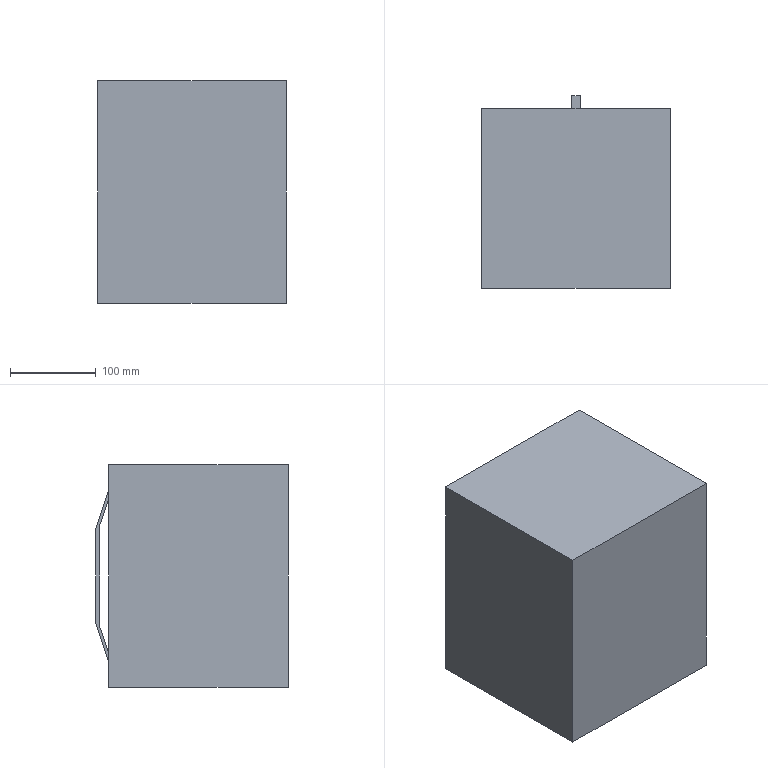Part | SolidWorks | features BaseBody 1 | 1 solid | 14 faces | box 220 x 225 x 260 mm | volume 12020250 mm3 | plane 14
STEP:
#1=CARTESIAN_POINT('',(-5.,120.,55.));
#2=VERTEX_POINT('',#1);
#3=CARTESIAN_POINT('',(5.,120.,55.));
#4=VERTEX_POINT('',#3);
#5=CARTESIAN_POINT('',(5.,120.,55.));
#6=DIRECTION('',(1.,0.,0.));
#7=VECTOR('',#6,1000.);
#8=LINE('',#5,#7);
#9=EDGE_CURVE('',#2,#4,#8,.T.);
#10=ORIENTED_EDGE('',*,*,#9,.T.);
#11=CARTESIAN_POINT('',(5.,120.,-55.));
#12=VERTEX_POINT('',#11);
#13=CARTESIAN_POINT('',(5.,120.,0.));
#14=DIRECTION('',(0.,0.,-1.));
#15=VECTOR('',#14,1000.);
#16=LINE('',#13,#15);
#17=EDGE_CURVE('',#4,#12,#16,.T.);
#18=ORIENTED_EDGE('',*,*,#17,.T.);
#19=CARTESIAN_POINT('',(-5.,120.,-55.));
#20=VERTEX_POINT('',#19);
#21=CARTESIAN_POINT('',(5.,120.,-55.));
#22=DIRECTION('',(-1.,0.,0.));
#23=VECTOR('',#22,1000.);
#24=LINE('',#21,#23);
#25=EDGE_CURVE('',#12,#20,#24,.T.);
#26=ORIENTED_EDGE('',*,*,#25,.T.);
#27=CARTESIAN_POINT('',(-5.,120.,0.));
#28=DIRECTION('',(0.,0.,-1.));
#29=VECTOR('',#28,1000.);
#30=LINE('',#27,#29);
#31=EDGE_CURVE('',#2,#20,#30,.T.);
#32=ORIENTED_EDGE('',*,*,#31,.F.);
#33=EDGE_LOOP('',(#10,#18,#26,#32));
#34=FACE_OUTER_BOUND('',#33,.T.);
#35=CARTESIAN_POINT('',(5.,120.,55.));
#36=DIRECTION('',(0.,-1.,0.));
#37=DIRECTION('',(0.,0.,-1.));
#38=AXIS2_PLACEMENT_3D('',#35,#36,#37);
#39=PLANE('',#38);
#40=ADVANCED_FACE('',(#34),#39,.F.);
#41=CARTESIAN_POINT('',(-5.,115.,-60.));
#42=VERTEX_POINT('',#41);
#43=CARTESIAN_POINT('',(5.,115.,-60.));
#44=VERTEX_POINT('',#43);
#45=CARTESIAN_POINT('',(5.,115.,-60.));
#46=DIRECTION('',(1.,0.,0.));
#47=VECTOR('',#46,1000.);
#48=LINE('',#45,#47);
#49=EDGE_CURVE('',#42,#44,#48,.T.);
#50=ORIENTED_EDGE('',*,*,#49,.T.);
#51=CARTESIAN_POINT('',(5.,115.,60.));
#52=VERTEX_POINT('',#51);
#53=CARTESIAN_POINT('',(5.,115.,0.));
#54=DIRECTION('',(0.,0.,1.));
#55=VECTOR('',#54,1000.);
#56=LINE('',#53,#55);
#57=EDGE_CURVE('',#44,#52,#56,.T.);
#58=ORIENTED_EDGE('',*,*,#57,.T.);
#59=CARTESIAN_POINT('',(-5.,115.,60.));
#60=VERTEX_POINT('',#59);
#61=CARTESIAN_POINT('',(5.,115.,60.));
#62=DIRECTION('',(-1.,0.,0.));
#63=VECTOR('',#62,1000.);
#64=LINE('',#61,#63);
#65=EDGE_CURVE('',#52,#60,#64,.T.);
#66=ORIENTED_EDGE('',*,*,#65,.T.);
#67=CARTESIAN_POINT('',(-5.,115.,0.));
#68=DIRECTION('',(0.,0.,1.));
#69=VECTOR('',#68,1000.);
#70=LINE('',#67,#69);
#71=EDGE_CURVE('',#42,#60,#70,.T.);
#72=ORIENTED_EDGE('',*,*,#71,.F.);
#73=EDGE_LOOP('',(#50,#58,#66,#72));
#74=FACE_OUTER_BOUND('',#73,.T.);
#75=CARTESIAN_POINT('',(5.,115.,-60.));
#76=DIRECTION('',(0.,1.,0.));
#77=DIRECTION('',(0.,0.,-1.));
#78=AXIS2_PLACEMENT_3D('',#75,#76,#77);
#79=PLANE('',#78);
#80=ADVANCED_FACE('',(#74),#79,.F.);
#81=ORIENTED_EDGE('',*,*,#25,.F.);
#82=CARTESIAN_POINT('',(5.,105.,-100.));
#83=VERTEX_POINT('',#82);
#84=CARTESIAN_POINT('',(5.,120.,-55.));
#85=DIRECTION('',(0.,-0.3162,-0.9487));
#86=VECTOR('',#85,1000.);
#87=LINE('',#84,#86);
#88=EDGE_CURVE('',#12,#83,#87,.T.);
#89=ORIENTED_EDGE('',*,*,#88,.T.);
#90=CARTESIAN_POINT('',(-5.,105.,-100.));
#91=VERTEX_POINT('',#90);
#92=CARTESIAN_POINT('',(-110.,105.,-100.));
#93=DIRECTION('',(-1.,0.,0.));
#94=VECTOR('',#93,1000.);
#95=LINE('',#92,#94);
#96=EDGE_CURVE('',#83,#91,#95,.T.);
#97=ORIENTED_EDGE('',*,*,#96,.T.);
#98=CARTESIAN_POINT('',(-5.,120.,-55.));
#99=DIRECTION('',(0.,-0.3162,-0.9487));
#100=VECTOR('',#99,1000.);
#101=LINE('',#98,#100);
#102=EDGE_CURVE('',#20,#91,#101,.T.);
#103=ORIENTED_EDGE('',*,*,#102,.F.);
#104=EDGE_LOOP('',(#81,#89,#97,#103));
#105=FACE_OUTER_BOUND('',#104,.T.);
#106=CARTESIAN_POINT('',(5.,120.,-55.));
#107=DIRECTION('',(0.,-0.9487,0.3162));
#108=DIRECTION('',(-1.,0.,0.));
#109=AXIS2_PLACEMENT_3D('',#106,#107,#108);
#110=PLANE('',#109);
#111=ADVANCED_FACE('',(#105),#110,.F.);
#112=CARTESIAN_POINT('',(-5.,105.,-90.));
#113=VERTEX_POINT('',#112);
#114=CARTESIAN_POINT('',(5.,105.,-90.));
#115=VERTEX_POINT('',#114);
#116=CARTESIAN_POINT('',(-110.,105.,-90.));
#117=DIRECTION('',(1.,0.,0.));
#118=VECTOR('',#117,1000.);
#119=LINE('',#116,#118);
#120=EDGE_CURVE('',#113,#115,#119,.T.);
#121=ORIENTED_EDGE('',*,*,#120,.T.);
#122=CARTESIAN_POINT('',(5.,105.,-90.));
#123=DIRECTION('',(0.,0.3162,0.9487));
#124=VECTOR('',#123,1000.);
#125=LINE('',#122,#124);
#126=EDGE_CURVE('',#115,#44,#125,.T.);
#127=ORIENTED_EDGE('',*,*,#126,.T.);
#128=ORIENTED_EDGE('',*,*,#49,.F.);
#129=CARTESIAN_POINT('',(-5.,105.,-90.));
#130=DIRECTION('',(0.,0.3162,0.9487));
#131=VECTOR('',#130,1000.);
#132=LINE('',#129,#131);
#133=EDGE_CURVE('',#113,#42,#132,.T.);
#134=ORIENTED_EDGE('',*,*,#133,.F.);
#135=EDGE_LOOP('',(#121,#127,#128,#134));
#136=FACE_OUTER_BOUND('',#135,.T.);
#137=CARTESIAN_POINT('',(5.,105.,-90.));
#138=DIRECTION('',(0.,0.9487,-0.3162));
#139=DIRECTION('',(-1.,0.,0.));
#140=AXIS2_PLACEMENT_3D('',#137,#138,#139);
#141=PLANE('',#140);
#142=ADVANCED_FACE('',(#136),#141,.F.);
#143=ORIENTED_EDGE('',*,*,#65,.F.);
#144=CARTESIAN_POINT('',(5.,105.,90.));
#145=VERTEX_POINT('',#144);
#146=CARTESIAN_POINT('',(5.,115.,60.));
#147=DIRECTION('',(0.,-0.3162,0.9487));
#148=VECTOR('',#147,1000.);
#149=LINE('',#146,#148);
#150=EDGE_CURVE('',#52,#145,#149,.T.);
#151=ORIENTED_EDGE('',*,*,#150,.T.);
#152=CARTESIAN_POINT('',(-5.,105.,90.));
#153=VERTEX_POINT('',#152);
#154=CARTESIAN_POINT('',(-110.,105.,90.));
#155=DIRECTION('',(-1.,0.,0.));
#156=VECTOR('',#155,1000.);
#157=LINE('',#154,#156);
#158=EDGE_CURVE('',#145,#153,#157,.T.);
#159=ORIENTED_EDGE('',*,*,#158,.T.);
#160=CARTESIAN_POINT('',(-5.,115.,60.));
#161=DIRECTION('',(0.,-0.3162,0.9487));
#162=VECTOR('',#161,1000.);
#163=LINE('',#160,#162);
#164=EDGE_CURVE('',#60,#153,#163,.T.);
#165=ORIENTED_EDGE('',*,*,#164,.F.);
#166=EDGE_LOOP('',(#143,#151,#159,#165));
#167=FACE_OUTER_BOUND('',#166,.T.);
#168=CARTESIAN_POINT('',(5.,115.,60.));
#169=DIRECTION('',(0.,0.9487,0.3162));
#170=DIRECTION('',(1.,0.,0.));
#171=AXIS2_PLACEMENT_3D('',#168,#169,#170);
#172=PLANE('',#171);
#173=ADVANCED_FACE('',(#167),#172,.F.);
#174=ORIENTED_EDGE('',*,*,#164,.T.);
#175=CARTESIAN_POINT('',(-5.,105.,100.));
#176=VERTEX_POINT('',#175);
#177=CARTESIAN_POINT('',(-5.,105.,130.));
#178=DIRECTION('',(0.,0.,1.));
#179=VECTOR('',#178,1000.);
#180=LINE('',#177,#179);
#181=EDGE_CURVE('',#153,#176,#180,.T.);
#182=ORIENTED_EDGE('',*,*,#181,.T.);
#183=CARTESIAN_POINT('',(-5.,105.,100.));
#184=DIRECTION('',(0.,0.3162,-0.9487));
#185=VECTOR('',#184,1000.);
#186=LINE('',#183,#185);
#187=EDGE_CURVE('',#176,#2,#186,.T.);
#188=ORIENTED_EDGE('',*,*,#187,.T.);
#189=ORIENTED_EDGE('',*,*,#31,.T.);
#190=ORIENTED_EDGE('',*,*,#102,.T.);
#191=CARTESIAN_POINT('',(-5.,105.,130.));
#192=DIRECTION('',(0.,0.,1.));
#193=VECTOR('',#192,1000.);
#194=LINE('',#191,#193);
#195=EDGE_CURVE('',#91,#113,#194,.T.);
#196=ORIENTED_EDGE('',*,*,#195,.T.);
#197=ORIENTED_EDGE('',*,*,#133,.T.);
#198=ORIENTED_EDGE('',*,*,#71,.T.);
#199=EDGE_LOOP('',(#174,#182,#188,#189,#190,#196,#197,#198));
#200=FACE_OUTER_BOUND('',#199,.T.);
#201=CARTESIAN_POINT('',(-5.,138.333,0.));
#202=DIRECTION('',(-1.,0.,0.));
#203=DIRECTION('',(0.,0.,1.));
#204=AXIS2_PLACEMENT_3D('',#201,#202,#203);
#205=PLANE('',#204);
#206=ADVANCED_FACE('',(#200),#205,.T.);
#207=CARTESIAN_POINT('',(5.,105.,100.));
#208=VERTEX_POINT('',#207);
#209=CARTESIAN_POINT('',(-110.,105.,100.));
#210=DIRECTION('',(1.,0.,0.));
#211=VECTOR('',#210,1000.);
#212=LINE('',#209,#211);
#213=EDGE_CURVE('',#176,#208,#212,.T.);
#214=ORIENTED_EDGE('',*,*,#213,.T.);
#215=CARTESIAN_POINT('',(5.,105.,100.));
#216=DIRECTION('',(0.,0.3162,-0.9487));
#217=VECTOR('',#216,1000.);
#218=LINE('',#215,#217);
#219=EDGE_CURVE('',#208,#4,#218,.T.);
#220=ORIENTED_EDGE('',*,*,#219,.T.);
#221=ORIENTED_EDGE('',*,*,#9,.F.);
#222=ORIENTED_EDGE('',*,*,#187,.F.);
#223=EDGE_LOOP('',(#214,#220,#221,#222));
#224=FACE_OUTER_BOUND('',#223,.T.);
#225=CARTESIAN_POINT('',(5.,105.,100.));
#226=DIRECTION('',(0.,-0.9487,-0.3162));
#227=DIRECTION('',(0.,0.3162,-0.9487));
#228=AXIS2_PLACEMENT_3D('',#225,#226,#227);
#229=PLANE('',#228);
#230=ADVANCED_FACE('',(#224),#229,.F.);
#231=CARTESIAN_POINT('',(5.,105.,130.));
#232=DIRECTION('',(0.,0.,-1.));
#233=VECTOR('',#232,1000.);
#234=LINE('',#231,#233);
#235=EDGE_CURVE('',#208,#145,#234,.T.);
#236=ORIENTED_EDGE('',*,*,#235,.T.);
#237=ORIENTED_EDGE('',*,*,#150,.F.);
#238=ORIENTED_EDGE('',*,*,#57,.F.);
#239=ORIENTED_EDGE('',*,*,#126,.F.);
#240=CARTESIAN_POINT('',(5.,105.,130.));
#241=DIRECTION('',(0.,0.,-1.));
#242=VECTOR('',#241,1000.);
#243=LINE('',#240,#242);
#244=EDGE_CURVE('',#115,#83,#243,.T.);
#245=ORIENTED_EDGE('',*,*,#244,.T.);
#246=ORIENTED_EDGE('',*,*,#88,.F.);
#247=ORIENTED_EDGE('',*,*,#17,.F.);
#248=ORIENTED_EDGE('',*,*,#219,.F.);
#249=EDGE_LOOP('',(#236,#237,#238,#239,#245,#246,#247,#248));
#250=FACE_OUTER_BOUND('',#249,.T.);
#251=CARTESIAN_POINT('',(5.,138.333,0.));
#252=DIRECTION('',(-1.,0.,0.));
#253=DIRECTION('',(0.,0.,1.));
#254=AXIS2_PLACEMENT_3D('',#251,#252,#253);
#255=PLANE('',#254);
#256=ADVANCED_FACE('',(#250),#255,.F.);
#257=ORIENTED_EDGE('',*,*,#120,.F.);
#258=ORIENTED_EDGE('',*,*,#195,.F.);
#259=ORIENTED_EDGE('',*,*,#96,.F.);
#260=ORIENTED_EDGE('',*,*,#244,.F.);
#261=EDGE_LOOP('',(#257,#258,#259,#260));
#262=FACE_BOUND('',#261,.T.);
#263=ORIENTED_EDGE('',*,*,#213,.F.);
#264=ORIENTED_EDGE('',*,*,#181,.F.);
#265=ORIENTED_EDGE('',*,*,#158,.F.);
#266=ORIENTED_EDGE('',*,*,#235,.F.);
#267=EDGE_LOOP('',(#263,#264,#265,#266));
#268=FACE_BOUND('',#267,.T.);
#269=CARTESIAN_POINT('',(-110.,105.,-130.));
#270=VERTEX_POINT('',#269);
#271=CARTESIAN_POINT('',(-110.,105.,130.));
#272=VERTEX_POINT('',#271);
#273=CARTESIAN_POINT('',(-110.,105.,130.));
#274=DIRECTION('',(0.,0.,1.));
#275=VECTOR('',#274,1000.);
#276=LINE('',#273,#275);
#277=EDGE_CURVE('',#270,#272,#276,.T.);
#278=ORIENTED_EDGE('',*,*,#277,.T.);
#279=CARTESIAN_POINT('',(110.,105.,130.));
#280=VERTEX_POINT('',#279);
#281=CARTESIAN_POINT('',(110.,105.,130.));
#282=DIRECTION('',(-1.,0.,0.));
#283=VECTOR('',#282,1000.);
#284=LINE('',#281,#283);
#285=EDGE_CURVE('',#280,#272,#284,.T.);
#286=ORIENTED_EDGE('',*,*,#285,.F.);
#287=CARTESIAN_POINT('',(110.,105.,-130.));
#288=VERTEX_POINT('',#287);
#289=CARTESIAN_POINT('',(110.,105.,130.));
#290=DIRECTION('',(0.,0.,-1.));
#291=VECTOR('',#290,1000.);
#292=LINE('',#289,#291);
#293=EDGE_CURVE('',#280,#288,#292,.T.);
#294=ORIENTED_EDGE('',*,*,#293,.T.);
#295=CARTESIAN_POINT('',(110.,105.,-130.));
#296=DIRECTION('',(-1.,0.,0.));
#297=VECTOR('',#296,1000.);
#298=LINE('',#295,#297);
#299=EDGE_CURVE('',#288,#270,#298,.T.);
#300=ORIENTED_EDGE('',*,*,#299,.T.);
#301=EDGE_LOOP('',(#278,#286,#294,#300));
#302=FACE_OUTER_BOUND('',#301,.T.);
#303=CARTESIAN_POINT('',(-110.,105.,130.));
#304=DIRECTION('',(0.,-1.,0.));
#305=DIRECTION('',(0.,0.,-1.));
#306=AXIS2_PLACEMENT_3D('',#303,#304,#305);
#307=PLANE('',#306);
#308=ADVANCED_FACE('',(#262,#268,#302),#307,.F.);
#309=CARTESIAN_POINT('',(-110.,-105.,-130.));
#310=VERTEX_POINT('',#309);
#311=CARTESIAN_POINT('',(-110.,-105.,130.));
#312=VERTEX_POINT('',#311);
#313=CARTESIAN_POINT('',(-110.,-105.,130.));
#314=DIRECTION('',(0.,0.,1.));
#315=VECTOR('',#314,1000.);
#316=LINE('',#313,#315);
#317=EDGE_CURVE('',#310,#312,#316,.T.);
#318=ORIENTED_EDGE('',*,*,#317,.T.);
#319=CARTESIAN_POINT('',(-110.,-105.,130.));
#320=DIRECTION('',(0.,-1.,0.));
#321=VECTOR('',#320,1000.);
#322=LINE('',#319,#321);
#323=EDGE_CURVE('',#272,#312,#322,.T.);
#324=ORIENTED_EDGE('',*,*,#323,.F.);
#325=ORIENTED_EDGE('',*,*,#277,.F.);
#326=CARTESIAN_POINT('',(-110.,-105.,-130.));
#327=DIRECTION('',(0.,-1.,0.));
#328=VECTOR('',#327,1000.);
#329=LINE('',#326,#328);
#330=EDGE_CURVE('',#270,#310,#329,.T.);
#331=ORIENTED_EDGE('',*,*,#330,.T.);
#332=EDGE_LOOP('',(#318,#324,#325,#331));
#333=FACE_OUTER_BOUND('',#332,.T.);
#334=CARTESIAN_POINT('',(-110.,105.,130.));
#335=DIRECTION('',(1.,0.,0.));
#336=DIRECTION('',(0.,1.,0.));
#337=AXIS2_PLACEMENT_3D('',#334,#335,#336);
#338=PLANE('',#337);
#339=ADVANCED_FACE('',(#333),#338,.F.);
#340=ORIENTED_EDGE('',*,*,#323,.T.);
#341=CARTESIAN_POINT('',(110.,-105.,130.));
#342=VERTEX_POINT('',#341);
#343=CARTESIAN_POINT('',(-110.,-105.,130.));
#344=DIRECTION('',(1.,0.,0.));
#345=VECTOR('',#344,1000.);
#346=LINE('',#343,#345);
#347=EDGE_CURVE('',#312,#342,#346,.T.);
#348=ORIENTED_EDGE('',*,*,#347,.T.);
#349=CARTESIAN_POINT('',(110.,105.,130.));
#350=DIRECTION('',(0.,1.,0.));
#351=VECTOR('',#350,1000.);
#352=LINE('',#349,#351);
#353=EDGE_CURVE('',#342,#280,#352,.T.);
#354=ORIENTED_EDGE('',*,*,#353,.T.);
#355=ORIENTED_EDGE('',*,*,#285,.T.);
#356=EDGE_LOOP('',(#340,#348,#354,#355));
#357=FACE_OUTER_BOUND('',#356,.T.);
#358=CARTESIAN_POINT('',(110.,-105.,130.));
#359=DIRECTION('',(0.,0.,1.));
#360=DIRECTION('',(1.,0.,0.));
#361=AXIS2_PLACEMENT_3D('',#358,#359,#360);
#362=PLANE('',#361);
#363=ADVANCED_FACE('',(#357),#362,.T.);
#364=ORIENTED_EDGE('',*,*,#293,.F.);
#365=ORIENTED_EDGE('',*,*,#353,.F.);
#366=CARTESIAN_POINT('',(110.,-105.,-130.));
#367=VERTEX_POINT('',#366);
#368=CARTESIAN_POINT('',(110.,-105.,130.));
#369=DIRECTION('',(0.,0.,-1.));
#370=VECTOR('',#369,1000.);
#371=LINE('',#368,#370);
#372=EDGE_CURVE('',#342,#367,#371,.T.);
#373=ORIENTED_EDGE('',*,*,#372,.T.);
#374=CARTESIAN_POINT('',(110.,-105.,-130.));
#375=DIRECTION('',(0.,1.,0.));
#376=VECTOR('',#375,1000.);
#377=LINE('',#374,#376);
#378=EDGE_CURVE('',#367,#288,#377,.T.);
#379=ORIENTED_EDGE('',*,*,#378,.T.);
#380=EDGE_LOOP('',(#364,#365,#373,#379));
#381=FACE_OUTER_BOUND('',#380,.T.);
#382=CARTESIAN_POINT('',(110.,105.,130.));
#383=DIRECTION('',(-1.,0.,0.));
#384=DIRECTION('',(0.,1.,0.));
#385=AXIS2_PLACEMENT_3D('',#382,#383,#384);
#386=PLANE('',#385);
#387=ADVANCED_FACE('',(#381),#386,.F.);
#388=CARTESIAN_POINT('',(-110.,-105.,-130.));
#389=DIRECTION('',(-1.,0.,0.));
#390=VECTOR('',#389,1000.);
#391=LINE('',#388,#390);
#392=EDGE_CURVE('',#367,#310,#391,.T.);
#393=ORIENTED_EDGE('',*,*,#392,.T.);
#394=ORIENTED_EDGE('',*,*,#330,.F.);
#395=ORIENTED_EDGE('',*,*,#299,.F.);
#396=ORIENTED_EDGE('',*,*,#378,.F.);
#397=EDGE_LOOP('',(#393,#394,#395,#396));
#398=FACE_OUTER_BOUND('',#397,.T.);
#399=CARTESIAN_POINT('',(110.,-105.,-130.));
#400=DIRECTION('',(0.,0.,1.));
#401=DIRECTION('',(1.,0.,0.));
#402=AXIS2_PLACEMENT_3D('',#399,#400,#401);
#403=PLANE('',#402);
#404=ADVANCED_FACE('',(#398),#403,.F.);
#405=ORIENTED_EDGE('',*,*,#372,.F.);
#406=ORIENTED_EDGE('',*,*,#347,.F.);
#407=ORIENTED_EDGE('',*,*,#317,.F.);
#408=ORIENTED_EDGE('',*,*,#392,.F.);
#409=EDGE_LOOP('',(#405,#406,#407,#408));
#410=FACE_OUTER_BOUND('',#409,.T.);
#411=CARTESIAN_POINT('',(-110.,-105.,130.));
#412=DIRECTION('',(0.,1.,0.));
#413=DIRECTION('',(1.,0.,0.));
#414=AXIS2_PLACEMENT_3D('',#411,#412,#413);
#415=PLANE('',#414);
#416=ADVANCED_FACE('',(#410),#415,.F.);
#417=CLOSED_SHELL('',(#40,#80,#111,#142,#173,#206,#230,#256,#308,#339,#363,#387,#404,#416));
#418=MANIFOLD_SOLID_BREP('',#417);
#419=CARTESIAN_POINT('',(0.,0.,0.));
#420=DIRECTION('',(0.,0.,1.));
#421=DIRECTION('',(1.,0.,0.));
#422=AXIS2_PLACEMENT_3D('',#419,#420,#421);
#423=(LENGTH_UNIT()NAMED_UNIT(*)SI_UNIT(.MILLI.,.METRE.));
#424=UNCERTAINTY_MEASURE_WITH_UNIT(LENGTH_MEASURE(0.00001),#423,'','');
#425=(NAMED_UNIT(*)PLANE_ANGLE_UNIT()SI_UNIT($,.RADIAN.));
#426=(NAMED_UNIT(*)SI_UNIT($,.STERADIAN.)SOLID_ANGLE_UNIT());
#427=(GEOMETRIC_REPRESENTATION_CONTEXT(3)GLOBAL_UNCERTAINTY_ASSIGNED_CONTEXT((#424))GLOBAL_UNIT_ASSIGNED_CONTEXT((#423,#425,#426))REPRESENTATION_CONTEXT('',''));
#428=ADVANCED_BREP_SHAPE_REPRESENTATION('',(#418,#422),#427);